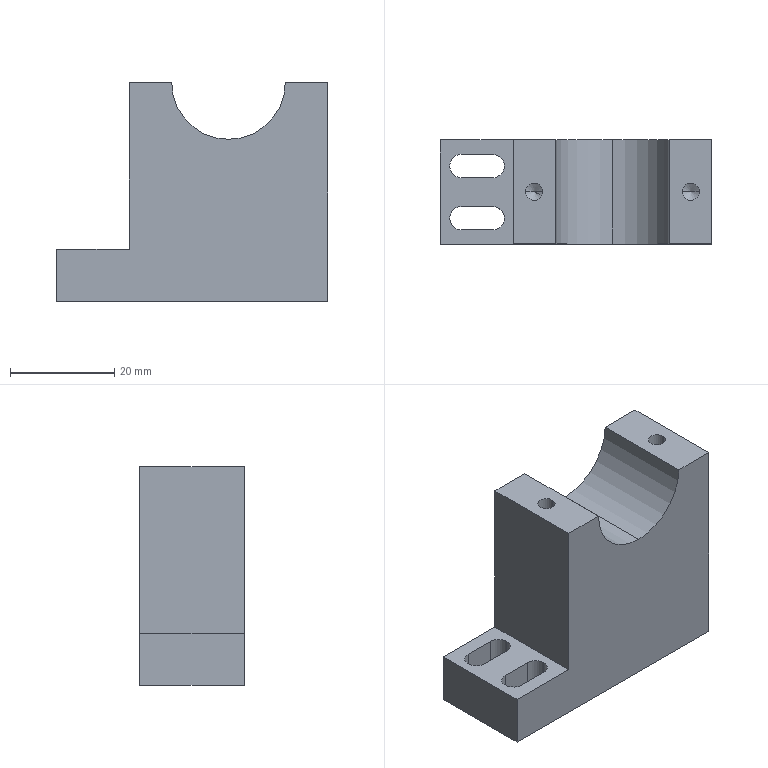Part | STEP file | PN_0083 Mount electronic clip cylinder fixed support seat A | 1 solid | 29 faces | box 52 x 20 x 42 mm | volume 29893 mm3 | plane 13 | cylinder 12 | cone 4 | commonest cylinder face diameters 4.5 x6 3.3 x4 21.8 x2